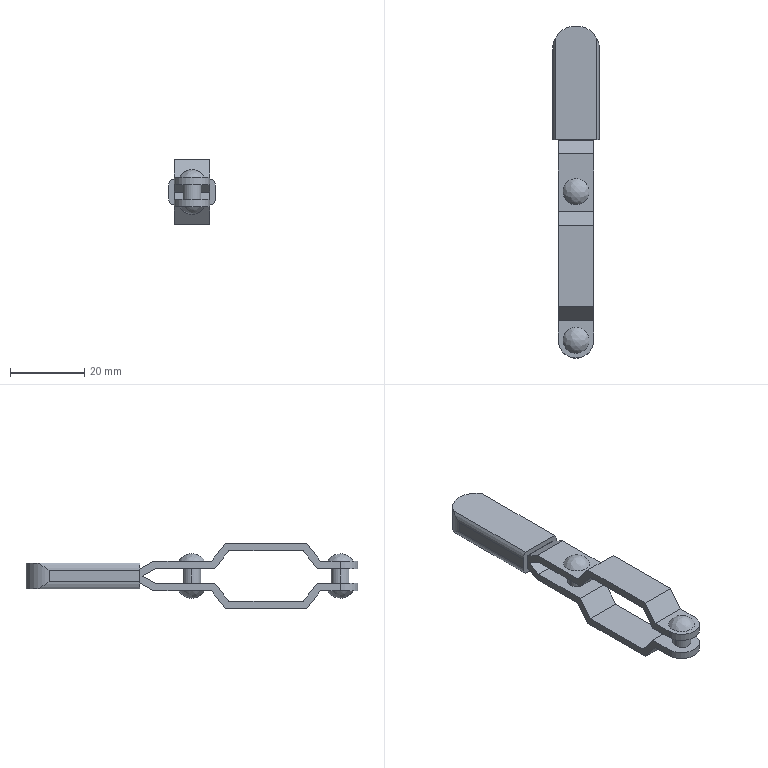Part | SolidWorks | features BaseBody 1 | 1 solid | 48 faces | box 12.6 x 89.5 x 17.6 mm | volume 5262 mm3 | plane 33 | cylinder 11 | spline 4 | commonest cylinder face diameters 4.8 x4 6 x4 9.6 x2 12.6 x1